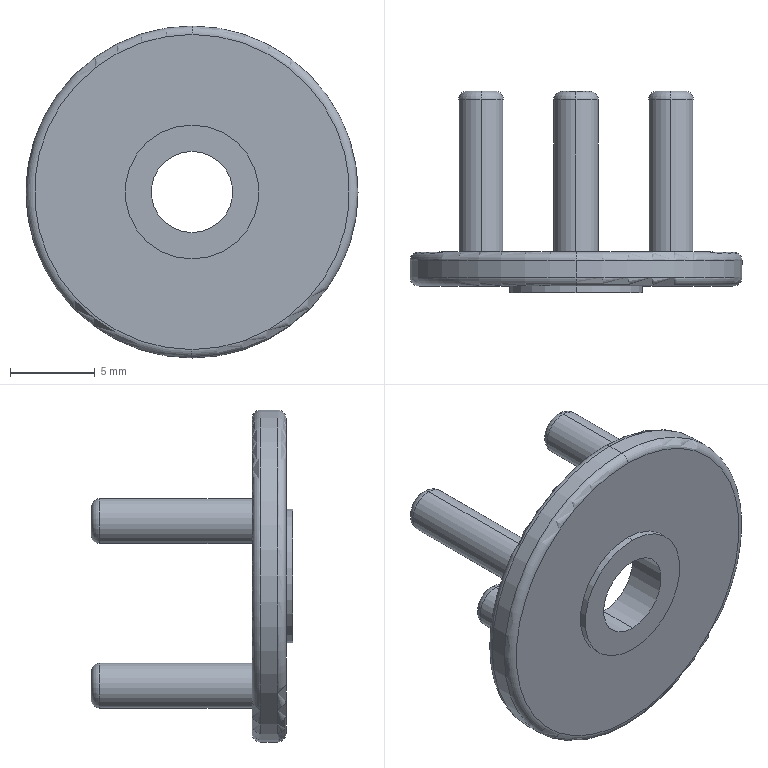Part | SolidWorks | features BaseBody 1 | 1 solid | 28 faces | box 19.6 x 11.9 x 19.6 mm | volume 729.046 mm3 | cylinder 12 | torus 10 | plane 6 | commonest cylinder face diameters 2.65 x6 4.8 x2 7.9 x2 19.6 x2
STEP:
#1=CARTESIAN_POINT('',(0.,0.,3.95));
#2=VERTEX_POINT('',#1);
#3=CARTESIAN_POINT('',(0.,0.,-3.95));
#4=VERTEX_POINT('',#3);
#5=CARTESIAN_POINT('',(0.,0.,0.));
#6=DIRECTION('',(0.,1.,0.));
#7=DIRECTION('',(0.,0.,1.));
#8=AXIS2_PLACEMENT_3D('',#5,#6,#7);
#9=CIRCLE('',#8,3.95);
#10=EDGE_CURVE('',#2,#4,#9,.T.);
#11=ORIENTED_EDGE('',*,*,#10,.F.);
#12=CARTESIAN_POINT('',(0.,-0.4,3.95));
#13=VERTEX_POINT('',#12);
#14=CARTESIAN_POINT('',(0.,-0.4,3.95));
#15=DIRECTION('',(0.,1.,0.));
#16=VECTOR('',#15,1000.);
#17=LINE('',#14,#16);
#18=EDGE_CURVE('',#13,#2,#17,.T.);
#19=ORIENTED_EDGE('',*,*,#18,.F.);
#20=CARTESIAN_POINT('',(0.,-0.4,-3.95));
#21=VERTEX_POINT('',#20);
#22=CARTESIAN_POINT('',(0.,-0.4,0.));
#23=DIRECTION('',(0.,-1.,0.));
#24=DIRECTION('',(0.,0.,-1.));
#25=AXIS2_PLACEMENT_3D('',#22,#23,#24);
#26=CIRCLE('',#25,3.95);
#27=EDGE_CURVE('',#21,#13,#26,.T.);
#28=ORIENTED_EDGE('',*,*,#27,.F.);
#29=CARTESIAN_POINT('',(0.,0.,-3.95));
#30=DIRECTION('',(0.,-1.,0.));
#31=VECTOR('',#30,1000.);
#32=LINE('',#29,#31);
#33=EDGE_CURVE('',#4,#21,#32,.T.);
#34=ORIENTED_EDGE('',*,*,#33,.F.);
#35=EDGE_LOOP('',(#11,#19,#28,#34));
#36=FACE_OUTER_BOUND('',#35,.T.);
#37=CARTESIAN_POINT('',(0.,-0.4,0.));
#38=DIRECTION('',(0.,1.,0.));
#39=DIRECTION('',(0.,0.,1.));
#40=AXIS2_PLACEMENT_3D('',#37,#38,#39);
#41=CYLINDRICAL_SURFACE('',#40,3.95);
#42=ADVANCED_FACE('',(#36),#41,.T.);
#43=ORIENTED_EDGE('',*,*,#33,.T.);
#44=CARTESIAN_POINT('',(0.,-0.4,0.));
#45=DIRECTION('',(0.,-1.,0.));
#46=DIRECTION('',(0.,0.,1.));
#47=AXIS2_PLACEMENT_3D('',#44,#45,#46);
#48=CIRCLE('',#47,3.95);
#49=EDGE_CURVE('',#13,#21,#48,.T.);
#50=ORIENTED_EDGE('',*,*,#49,.F.);
#51=ORIENTED_EDGE('',*,*,#18,.T.);
#52=CARTESIAN_POINT('',(0.,0.,0.));
#53=DIRECTION('',(0.,1.,0.));
#54=DIRECTION('',(0.,0.,-1.));
#55=AXIS2_PLACEMENT_3D('',#52,#53,#54);
#56=CIRCLE('',#55,3.95);
#57=EDGE_CURVE('',#4,#2,#56,.T.);
#58=ORIENTED_EDGE('',*,*,#57,.F.);
#59=EDGE_LOOP('',(#43,#50,#51,#58));
#60=FACE_OUTER_BOUND('',#59,.T.);
#61=CARTESIAN_POINT('',(0.,-0.4,0.));
#62=DIRECTION('',(0.,1.,0.));
#63=DIRECTION('',(0.,0.,1.));
#64=AXIS2_PLACEMENT_3D('',#61,#62,#63);
#65=CYLINDRICAL_SURFACE('',#64,3.95);
#66=ADVANCED_FACE('',(#60),#65,.T.);
#67=CARTESIAN_POINT('',(0.,-0.4,2.4));
#68=VERTEX_POINT('',#67);
#69=CARTESIAN_POINT('',(0.,-0.4,-2.4));
#70=VERTEX_POINT('',#69);
#71=CARTESIAN_POINT('',(0.,-0.4,0.));
#72=DIRECTION('',(0.,-1.,0.));
#73=DIRECTION('',(0.,0.,1.));
#74=AXIS2_PLACEMENT_3D('',#71,#72,#73);
#75=CIRCLE('',#74,2.4);
#76=EDGE_CURVE('',#68,#70,#75,.T.);
#77=ORIENTED_EDGE('',*,*,#76,.F.);
#78=CARTESIAN_POINT('',(0.,-0.4,0.));
#79=DIRECTION('',(0.,-1.,0.));
#80=DIRECTION('',(0.,0.,-1.));
#81=AXIS2_PLACEMENT_3D('',#78,#79,#80);
#82=CIRCLE('',#81,2.4);
#83=EDGE_CURVE('',#70,#68,#82,.T.);
#84=ORIENTED_EDGE('',*,*,#83,.F.);
#85=EDGE_LOOP('',(#77,#84));
#86=FACE_BOUND('',#85,.T.);
#87=ORIENTED_EDGE('',*,*,#27,.T.);
#88=ORIENTED_EDGE('',*,*,#49,.T.);
#89=EDGE_LOOP('',(#87,#88));
#90=FACE_OUTER_BOUND('',#89,.T.);
#91=CARTESIAN_POINT('',(0.,-0.4,0.));
#92=DIRECTION('',(0.,-1.,0.));
#93=DIRECTION('',(0.,0.,-1.));
#94=AXIS2_PLACEMENT_3D('',#91,#92,#93);
#95=PLANE('',#94);
#96=ADVANCED_FACE('',(#86,#90),#95,.T.);
#97=CARTESIAN_POINT('',(0.,2.,9.3));
#98=VERTEX_POINT('',#97);
#99=CARTESIAN_POINT('',(0.,2.,-9.3));
#100=VERTEX_POINT('',#99);
#101=CARTESIAN_POINT('',(0.,2.,0.));
#102=DIRECTION('',(0.,1.,0.));
#103=DIRECTION('',(0.,0.,1.));
#104=AXIS2_PLACEMENT_3D('',#101,#102,#103);
#105=CIRCLE('',#104,9.3);
#106=EDGE_CURVE('',#98,#100,#105,.T.);
#107=ORIENTED_EDGE('',*,*,#106,.F.);
#108=CARTESIAN_POINT('',(0.,1.5,9.8));
#109=VERTEX_POINT('',#108);
#110=CARTESIAN_POINT('',(0.,1.5,9.3));
#111=DIRECTION('',(-1.,0.,0.));
#112=DIRECTION('',(0.,0.,1.));
#113=AXIS2_PLACEMENT_3D('',#110,#111,#112);
#114=CIRCLE('',#113,0.5);
#115=EDGE_CURVE('',#109,#98,#114,.T.);
#116=ORIENTED_EDGE('',*,*,#115,.F.);
#117=CARTESIAN_POINT('',(0.,1.5,-9.8));
#118=VERTEX_POINT('',#117);
#119=CARTESIAN_POINT('',(0.,1.5,0.));
#120=DIRECTION('',(0.,-1.,0.));
#121=DIRECTION('',(0.,0.,-1.));
#122=AXIS2_PLACEMENT_3D('',#119,#120,#121);
#123=CIRCLE('',#122,9.8);
#124=EDGE_CURVE('',#118,#109,#123,.T.);
#125=ORIENTED_EDGE('',*,*,#124,.F.);
#126=CARTESIAN_POINT('',(0.,1.5,-9.3));
#127=DIRECTION('',(-1.,0.,0.));
#128=DIRECTION('',(0.,1.,0.));
#129=AXIS2_PLACEMENT_3D('',#126,#127,#128);
#130=CIRCLE('',#129,0.5);
#131=EDGE_CURVE('',#100,#118,#130,.T.);
#132=ORIENTED_EDGE('',*,*,#131,.F.);
#133=EDGE_LOOP('',(#107,#116,#125,#132));
#134=FACE_OUTER_BOUND('',#133,.T.);
#135=CARTESIAN_POINT('',(0.,1.5,0.));
#136=DIRECTION('',(0.,-1.,0.));
#137=DIRECTION('',(0.,0.,1.));
#138=AXIS2_PLACEMENT_3D('',#135,#136,#137);
#139=TOROIDAL_SURFACE('',#138,9.3,0.5);
#140=ADVANCED_FACE('',(#134),#139,.T.);
#141=ORIENTED_EDGE('',*,*,#131,.T.);
#142=CARTESIAN_POINT('',(0.,1.5,0.));
#143=DIRECTION('',(0.,-1.,0.));
#144=DIRECTION('',(0.,0.,1.));
#145=AXIS2_PLACEMENT_3D('',#142,#143,#144);
#146=CIRCLE('',#145,9.8);
#147=EDGE_CURVE('',#109,#118,#146,.T.);
#148=ORIENTED_EDGE('',*,*,#147,.F.);
#149=ORIENTED_EDGE('',*,*,#115,.T.);
#150=CARTESIAN_POINT('',(0.,2.,0.));
#151=DIRECTION('',(0.,1.,0.));
#152=DIRECTION('',(0.,0.,-1.));
#153=AXIS2_PLACEMENT_3D('',#150,#151,#152);
#154=CIRCLE('',#153,9.3);
#155=EDGE_CURVE('',#100,#98,#154,.T.);
#156=ORIENTED_EDGE('',*,*,#155,.F.);
#157=EDGE_LOOP('',(#141,#148,#149,#156));
#158=FACE_OUTER_BOUND('',#157,.T.);
#159=CARTESIAN_POINT('',(0.,1.5,0.));
#160=DIRECTION('',(0.,-1.,0.));
#161=DIRECTION('',(0.,0.,1.));
#162=AXIS2_PLACEMENT_3D('',#159,#160,#161);
#163=TOROIDAL_SURFACE('',#162,9.3,0.5);
#164=ADVANCED_FACE('',(#158),#163,.T.);
#165=CARTESIAN_POINT('',(0.,0.5,9.8));
#166=VERTEX_POINT('',#165);
#167=CARTESIAN_POINT('',(0.,0.5,-9.8));
#168=VERTEX_POINT('',#167);
#169=CARTESIAN_POINT('',(0.,0.5,0.));
#170=DIRECTION('',(0.,1.,0.));
#171=DIRECTION('',(0.,0.,1.));
#172=AXIS2_PLACEMENT_3D('',#169,#170,#171);
#173=CIRCLE('',#172,9.8);
#174=EDGE_CURVE('',#166,#168,#173,.T.);
#175=ORIENTED_EDGE('',*,*,#174,.F.);
#176=CARTESIAN_POINT('',(0.,0.,9.3));
#177=VERTEX_POINT('',#176);
#178=CARTESIAN_POINT('',(0.,0.5,9.3));
#179=DIRECTION('',(-1.,0.,0.));
#180=DIRECTION('',(0.,-1.,0.00001628));
#181=AXIS2_PLACEMENT_3D('',#178,#179,#180);
#182=CIRCLE('',#181,0.5);
#183=EDGE_CURVE('',#177,#166,#182,.T.);
#184=ORIENTED_EDGE('',*,*,#183,.F.);
#185=CARTESIAN_POINT('',(0.,0.,-9.3));
#186=VERTEX_POINT('',#185);
#187=CARTESIAN_POINT('',(0.,0.,0.));
#188=DIRECTION('',(0.,-1.,0.));
#189=DIRECTION('',(0.,0.,-1.));
#190=AXIS2_PLACEMENT_3D('',#187,#188,#189);
#191=CIRCLE('',#190,9.3);
#192=EDGE_CURVE('',#186,#177,#191,.T.);
#193=ORIENTED_EDGE('',*,*,#192,.F.);
#194=CARTESIAN_POINT('',(0.,0.5,-9.3));
#195=DIRECTION('',(-1.,0.,0.));
#196=DIRECTION('',(0.,0.,-1.));
#197=AXIS2_PLACEMENT_3D('',#194,#195,#196);
#198=CIRCLE('',#197,0.5);
#199=EDGE_CURVE('',#168,#186,#198,.T.);
#200=ORIENTED_EDGE('',*,*,#199,.F.);
#201=EDGE_LOOP('',(#175,#184,#193,#200));
#202=FACE_OUTER_BOUND('',#201,.T.);
#203=CARTESIAN_POINT('',(0.,0.5,0.));
#204=DIRECTION('',(0.,-1.,0.));
#205=DIRECTION('',(0.,0.,1.));
#206=AXIS2_PLACEMENT_3D('',#203,#204,#205);
#207=TOROIDAL_SURFACE('',#206,9.3,0.5);
#208=ADVANCED_FACE('',(#202),#207,.T.);
#209=CARTESIAN_POINT('',(0.,0.5,0.));
#210=DIRECTION('',(0.,1.,0.));
#211=DIRECTION('',(0.,0.,-1.));
#212=AXIS2_PLACEMENT_3D('',#209,#210,#211);
#213=CIRCLE('',#212,9.8);
#214=EDGE_CURVE('',#168,#166,#213,.T.);
#215=ORIENTED_EDGE('',*,*,#214,.F.);
#216=ORIENTED_EDGE('',*,*,#199,.T.);
#217=CARTESIAN_POINT('',(0.,0.,0.));
#218=DIRECTION('',(0.,-1.,0.));
#219=DIRECTION('',(0.,0.,1.));
#220=AXIS2_PLACEMENT_3D('',#217,#218,#219);
#221=CIRCLE('',#220,9.3);
#222=EDGE_CURVE('',#177,#186,#221,.T.);
#223=ORIENTED_EDGE('',*,*,#222,.F.);
#224=ORIENTED_EDGE('',*,*,#183,.T.);
#225=EDGE_LOOP('',(#215,#216,#223,#224));
#226=FACE_OUTER_BOUND('',#225,.T.);
#227=CARTESIAN_POINT('',(0.,0.5,0.));
#228=DIRECTION('',(0.,-1.,0.));
#229=DIRECTION('',(0.,0.,1.));
#230=AXIS2_PLACEMENT_3D('',#227,#228,#229);
#231=TOROIDAL_SURFACE('',#230,9.3,0.5);
#232=ADVANCED_FACE('',(#226),#231,.T.);
#233=CARTESIAN_POINT('',(-5.608,11.5,4.062));
#234=VERTEX_POINT('',#233);
#235=CARTESIAN_POINT('',(-5.608,11.5,2.413));
#236=VERTEX_POINT('',#235);
#237=CARTESIAN_POINT('',(-5.608,11.5,3.237));
#238=DIRECTION('',(0.,1.,0.));
#239=DIRECTION('',(-0.000000017,0.,1.));
#240=AXIS2_PLACEMENT_3D('',#237,#238,#239);
#241=CIRCLE('',#240,0.825);
#242=EDGE_CURVE('',#234,#236,#241,.T.);
#243=ORIENTED_EDGE('',*,*,#242,.F.);
#244=CARTESIAN_POINT('',(-5.608,11.,4.562));
#245=VERTEX_POINT('',#244);
#246=CARTESIAN_POINT('',(-5.608,11.,4.062));
#247=DIRECTION('',(-1.,0.,0.));
#248=DIRECTION('',(0.,0.,1.));
#249=AXIS2_PLACEMENT_3D('',#246,#247,#248);
#250=CIRCLE('',#249,0.5);
#251=EDGE_CURVE('',#245,#234,#250,.T.);
#252=ORIENTED_EDGE('',*,*,#251,.F.);
#253=CARTESIAN_POINT('',(-5.608,11.,1.912));
#254=VERTEX_POINT('',#253);
#255=CARTESIAN_POINT('',(-5.608,11.,3.237));
#256=DIRECTION('',(0.,-1.,0.));
#257=DIRECTION('',(0.,0.,-1.));
#258=AXIS2_PLACEMENT_3D('',#255,#256,#257);
#259=CIRCLE('',#258,1.325);
#260=EDGE_CURVE('',#254,#245,#259,.T.);
#261=ORIENTED_EDGE('',*,*,#260,.F.);
#262=CARTESIAN_POINT('',(-5.608,11.,2.413));
#263=DIRECTION('',(-1.,0.,0.));
#264=DIRECTION('',(0.,1.,0.));
#265=AXIS2_PLACEMENT_3D('',#262,#263,#264);
#266=CIRCLE('',#265,0.5);
#267=EDGE_CURVE('',#236,#254,#266,.T.);
#268=ORIENTED_EDGE('',*,*,#267,.F.);
#269=EDGE_LOOP('',(#243,#252,#261,#268));
#270=FACE_OUTER_BOUND('',#269,.T.);
#271=CARTESIAN_POINT('',(-5.608,11.,3.237));
#272=DIRECTION('',(0.,-1.,0.));
#273=DIRECTION('',(0.,0.,1.));
#274=AXIS2_PLACEMENT_3D('',#271,#272,#273);
#275=TOROIDAL_SURFACE('',#274,0.825,0.5);
#276=ADVANCED_FACE('',(#270),#275,.T.);
#277=ORIENTED_EDGE('',*,*,#267,.T.);
#278=CARTESIAN_POINT('',(-5.608,11.,3.237));
#279=DIRECTION('',(0.,-1.,0.));
#280=DIRECTION('',(0.,0.,1.));
#281=AXIS2_PLACEMENT_3D('',#278,#279,#280);
#282=CIRCLE('',#281,1.325);
#283=EDGE_CURVE('',#245,#254,#282,.T.);
#284=ORIENTED_EDGE('',*,*,#283,.F.);
#285=ORIENTED_EDGE('',*,*,#251,.T.);
#286=CARTESIAN_POINT('',(-5.608,11.5,3.237));
#287=DIRECTION('',(0.,1.,0.));
#288=DIRECTION('',(0.,0.,-1.));
#289=AXIS2_PLACEMENT_3D('',#286,#287,#288);
#290=CIRCLE('',#289,0.825);
#291=EDGE_CURVE('',#236,#234,#290,.T.);
#292=ORIENTED_EDGE('',*,*,#291,.F.);
#293=EDGE_LOOP('',(#277,#284,#285,#292));
#294=FACE_OUTER_BOUND('',#293,.T.);
#295=CARTESIAN_POINT('',(-5.608,11.,3.237));
#296=DIRECTION('',(0.,-1.,0.));
#297=DIRECTION('',(0.,0.,1.));
#298=AXIS2_PLACEMENT_3D('',#295,#296,#297);
#299=TOROIDAL_SURFACE('',#298,0.825,0.5);
#300=ADVANCED_FACE('',(#294),#299,.T.);
#301=CARTESIAN_POINT('',(-0.000000007,11.5,-5.65));
#302=VERTEX_POINT('',#301);
#303=CARTESIAN_POINT('',(0.,11.5,-7.3));
#304=VERTEX_POINT('',#303);
#305=CARTESIAN_POINT('',(0.,11.5,-6.475));
#306=DIRECTION('',(0.,1.,0.));
#307=DIRECTION('',(-0.000000017,0.,1.));
#308=AXIS2_PLACEMENT_3D('',#305,#306,#307);
#309=CIRCLE('',#308,0.825);
#310=EDGE_CURVE('',#302,#304,#309,.T.);
#311=ORIENTED_EDGE('',*,*,#310,.F.);
#312=CARTESIAN_POINT('',(0.,11.,-5.15));
#313=VERTEX_POINT('',#312);
#314=CARTESIAN_POINT('',(0.,11.,-5.65));
#315=DIRECTION('',(-1.,0.,0.));
#316=DIRECTION('',(0.,0.,1.));
#317=AXIS2_PLACEMENT_3D('',#314,#315,#316);
#318=CIRCLE('',#317,0.5);
#319=EDGE_CURVE('',#313,#302,#318,.T.);
#320=ORIENTED_EDGE('',*,*,#319,.F.);
#321=CARTESIAN_POINT('',(0.,11.,-7.8));
#322=VERTEX_POINT('',#321);
#323=CARTESIAN_POINT('',(0.,11.,-6.475));
#324=DIRECTION('',(0.,-1.,0.));
#325=DIRECTION('',(0.,0.,-1.));
#326=AXIS2_PLACEMENT_3D('',#323,#324,#325);
#327=CIRCLE('',#326,1.325);
#328=EDGE_CURVE('',#322,#313,#327,.T.);
#329=ORIENTED_EDGE('',*,*,#328,.F.);
#330=CARTESIAN_POINT('',(0.,11.,-7.3));
#331=DIRECTION('',(-1.,0.,0.));
#332=DIRECTION('',(0.,1.,0.));
#333=AXIS2_PLACEMENT_3D('',#330,#331,#332);
#334=CIRCLE('',#333,0.5);
#335=EDGE_CURVE('',#304,#322,#334,.T.);
#336=ORIENTED_EDGE('',*,*,#335,.F.);
#337=EDGE_LOOP('',(#311,#320,#329,#336));
#338=FACE_OUTER_BOUND('',#337,.T.);
#339=CARTESIAN_POINT('',(0.,11.,-6.475));
#340=DIRECTION('',(0.,-1.,0.));
#341=DIRECTION('',(0.,0.,1.));
#342=AXIS2_PLACEMENT_3D('',#339,#340,#341);
#343=TOROIDAL_SURFACE('',#342,0.825,0.5);
#344=ADVANCED_FACE('',(#338),#343,.T.);
#345=ORIENTED_EDGE('',*,*,#335,.T.);
#346=CARTESIAN_POINT('',(0.,11.,-6.475));
#347=DIRECTION('',(0.,-1.,0.));
#348=DIRECTION('',(0.,0.,1.));
#349=AXIS2_PLACEMENT_3D('',#346,#347,#348);
#350=CIRCLE('',#349,1.325);
#351=EDGE_CURVE('',#313,#322,#350,.T.);
#352=ORIENTED_EDGE('',*,*,#351,.F.);
#353=ORIENTED_EDGE('',*,*,#319,.T.);
#354=CARTESIAN_POINT('',(0.,11.5,-6.475));
#355=DIRECTION('',(0.,1.,0.));
#356=DIRECTION('',(0.,0.,-1.));
#357=AXIS2_PLACEMENT_3D('',#354,#355,#356);
#358=CIRCLE('',#357,0.825);
#359=EDGE_CURVE('',#304,#302,#358,.T.);
#360=ORIENTED_EDGE('',*,*,#359,.F.);
#361=EDGE_LOOP('',(#345,#352,#353,#360));
#362=FACE_OUTER_BOUND('',#361,.T.);
#363=CARTESIAN_POINT('',(0.,11.,-6.475));
#364=DIRECTION('',(0.,-1.,0.));
#365=DIRECTION('',(0.,0.,1.));
#366=AXIS2_PLACEMENT_3D('',#363,#364,#365);
#367=TOROIDAL_SURFACE('',#366,0.825,0.5);
#368=ADVANCED_FACE('',(#362),#367,.T.);
#369=CARTESIAN_POINT('',(5.608,11.5,4.062));
#370=VERTEX_POINT('',#369);
#371=CARTESIAN_POINT('',(5.608,11.5,2.413));
#372=VERTEX_POINT('',#371);
#373=CARTESIAN_POINT('',(5.608,11.5,3.237));
#374=DIRECTION('',(0.,1.,0.));
#375=DIRECTION('',(-0.000000017,0.,1.));
#376=AXIS2_PLACEMENT_3D('',#373,#374,#375);
#377=CIRCLE('',#376,0.825);
#378=EDGE_CURVE('',#370,#372,#377,.T.);
#379=ORIENTED_EDGE('',*,*,#378,.F.);
#380=CARTESIAN_POINT('',(5.608,11.,4.562));
#381=VERTEX_POINT('',#380);
#382=CARTESIAN_POINT('',(5.608,11.,4.062));
#383=DIRECTION('',(-1.,0.,0.));
#384=DIRECTION('',(0.,0.,1.));
#385=AXIS2_PLACEMENT_3D('',#382,#383,#384);
#386=CIRCLE('',#385,0.5);
#387=EDGE_CURVE('',#381,#370,#386,.T.);
#388=ORIENTED_EDGE('',*,*,#387,.F.);
#389=CARTESIAN_POINT('',(5.608,11.,1.912));
#390=VERTEX_POINT('',#389);
#391=CARTESIAN_POINT('',(5.608,11.,3.237));
#392=DIRECTION('',(0.,-1.,0.));
#393=DIRECTION('',(0.,0.,-1.));
#394=AXIS2_PLACEMENT_3D('',#391,#392,#393);
#395=CIRCLE('',#394,1.325);
#396=EDGE_CURVE('',#390,#381,#395,.T.);
#397=ORIENTED_EDGE('',*,*,#396,.F.);
#398=CARTESIAN_POINT('',(5.608,11.,2.413));
#399=DIRECTION('',(-1.,0.,0.));
#400=DIRECTION('',(0.,1.,0.));
#401=AXIS2_PLACEMENT_3D('',#398,#399,#400);
#402=CIRCLE('',#401,0.5);
#403=EDGE_CURVE('',#372,#390,#402,.T.);
#404=ORIENTED_EDGE('',*,*,#403,.F.);
#405=EDGE_LOOP('',(#379,#388,#397,#404));
#406=FACE_OUTER_BOUND('',#405,.T.);
#407=CARTESIAN_POINT('',(5.608,11.,3.237));
#408=DIRECTION('',(0.,-1.,0.));
#409=DIRECTION('',(0.,0.,1.));
#410=AXIS2_PLACEMENT_3D('',#407,#408,#409);
#411=TOROIDAL_SURFACE('',#410,0.825,0.5);
#412=ADVANCED_FACE('',(#406),#411,.T.);
#413=ORIENTED_EDGE('',*,*,#403,.T.);
#414=CARTESIAN_POINT('',(5.608,11.,3.237));
#415=DIRECTION('',(0.,-1.,0.));
#416=DIRECTION('',(0.,0.,1.));
#417=AXIS2_PLACEMENT_3D('',#414,#415,#416);
#418=CIRCLE('',#417,1.325);
#419=EDGE_CURVE('',#381,#390,#418,.T.);
#420=ORIENTED_EDGE('',*,*,#419,.F.);
#421=ORIENTED_EDGE('',*,*,#387,.T.);
#422=CARTESIAN_POINT('',(5.608,11.5,3.237));
#423=DIRECTION('',(0.,1.,0.));
#424=DIRECTION('',(0.,0.,-1.));
#425=AXIS2_PLACEMENT_3D('',#422,#423,#424);
#426=CIRCLE('',#425,0.825);
#427=EDGE_CURVE('',#372,#370,#426,.T.);
#428=ORIENTED_EDGE('',*,*,#427,.F.);
#429=EDGE_LOOP('',(#413,#420,#421,#428));
#430=FACE_OUTER_BOUND('',#429,.T.);
#431=CARTESIAN_POINT('',(5.608,11.,3.237));
#432=DIRECTION('',(0.,-1.,0.));
#433=DIRECTION('',(0.,0.,1.));
#434=AXIS2_PLACEMENT_3D('',#431,#432,#433);
#435=TOROIDAL_SURFACE('',#434,0.825,0.5);
#436=ADVANCED_FACE('',(#430),#435,.T.);
#437=ORIENTED_EDGE('',*,*,#427,.T.);
#438=ORIENTED_EDGE('',*,*,#378,.T.);
#439=EDGE_LOOP('',(#437,#438));
#440=FACE_OUTER_BOUND('',#439,.T.);
#441=CARTESIAN_POINT('',(5.608,11.5,3.237));
#442=DIRECTION('',(0.,1.,0.));
#443=DIRECTION('',(1.,0.,0.));
#444=AXIS2_PLACEMENT_3D('',#441,#442,#443);
#445=PLANE('',#444);
#446=ADVANCED_FACE('',(#440),#445,.T.);
#447=CARTESIAN_POINT('',(5.608,2.,1.912));
#448=VERTEX_POINT('',#447);
#449=CARTESIAN_POINT('',(5.608,2.,4.562));
#450=VERTEX_POINT('',#449);
#451=CARTESIAN_POINT('',(5.608,2.,3.237));
#452=DIRECTION('',(0.,-1.,0.));
#453=DIRECTION('',(0.,0.,-1.));
#454=AXIS2_PLACEMENT_3D('',#451,#452,#453);
#455=CIRCLE('',#454,1.325);
#456=EDGE_CURVE('',#448,#450,#455,.T.);
#457=ORIENTED_EDGE('',*,*,#456,.F.);
#458=CARTESIAN_POINT('',(5.608,11.,1.912));
#459=DIRECTION('',(0.,-1.,0.));
#460=VECTOR('',#459,1000.);
#461=LINE('',#458,#460);
#462=EDGE_CURVE('',#390,#448,#461,.T.);
#463=ORIENTED_EDGE('',*,*,#462,.F.);
#464=ORIENTED_EDGE('',*,*,#396,.T.);
#465=CARTESIAN_POINT('',(5.608,2.,4.562));
#466=DIRECTION('',(0.,1.,0.));
#467=VECTOR('',#466,1000.);
#468=LINE('',#465,#467);
#469=EDGE_CURVE('',#450,#381,#468,.T.);
#470=ORIENTED_EDGE('',*,*,#469,.F.);
#471=EDGE_LOOP('',(#457,#463,#464,#470));
#472=FACE_OUTER_BOUND('',#471,.T.);
#473=CARTESIAN_POINT('',(5.608,11.,3.237));
#474=DIRECTION('',(0.,-1.,0.));
#475=DIRECTION('',(0.,0.,-1.));
#476=AXIS2_PLACEMENT_3D('',#473,#474,#475);
#477=CYLINDRICAL_SURFACE('',#476,1.325);
#478=ADVANCED_FACE('',(#472),#477,.T.);
#479=ORIENTED_EDGE('',*,*,#469,.T.);
#480=ORIENTED_EDGE('',*,*,#419,.T.);
#481=ORIENTED_EDGE('',*,*,#462,.T.);
#482=CARTESIAN_POINT('',(5.608,2.,3.237));
#483=DIRECTION('',(0.,-1.,0.));
#484=DIRECTION('',(0.,0.,1.));
#485=AXIS2_PLACEMENT_3D('',#482,#483,#484);
#486=CIRCLE('',#485,1.325);
#487=EDGE_CURVE('',#450,#448,#486,.T.);
#488=ORIENTED_EDGE('',*,*,#487,.F.);
#489=EDGE_LOOP('',(#479,#480,#481,#488));
#490=FACE_OUTER_BOUND('',#489,.T.);
#491=CARTESIAN_POINT('',(5.608,11.,3.237));
#492=DIRECTION('',(0.,-1.,0.));
#493=DIRECTION('',(0.,0.,-1.));
#494=AXIS2_PLACEMENT_3D('',#491,#492,#493);
#495=CYLINDRICAL_SURFACE('',#494,1.325);
#496=ADVANCED_FACE('',(#490),#495,.T.);
#497=ORIENTED_EDGE('',*,*,#291,.T.);
#498=ORIENTED_EDGE('',*,*,#242,.T.);
#499=EDGE_LOOP('',(#497,#498));
#500=FACE_OUTER_BOUND('',#499,.T.);
#501=CARTESIAN_POINT('',(-5.608,11.5,3.237));
#502=DIRECTION('',(0.,1.,0.));
#503=DIRECTION('',(1.,0.,0.));
#504=AXIS2_PLACEMENT_3D('',#501,#502,#503);
#505=PLANE('',#504);
#506=ADVANCED_FACE('',(#500),#505,.T.);
#507=CARTESIAN_POINT('',(-5.608,2.,1.912));
#508=VERTEX_POINT('',#507);
#509=CARTESIAN_POINT('',(-5.608,2.,4.562));
#510=VERTEX_POINT('',#509);
#511=CARTESIAN_POINT('',(-5.608,2.,3.237));
#512=DIRECTION('',(0.,-1.,0.));
#513=DIRECTION('',(0.,0.,-1.));
#514=AXIS2_PLACEMENT_3D('',#511,#512,#513);
#515=CIRCLE('',#514,1.325);
#516=EDGE_CURVE('',#508,#510,#515,.T.);
#517=ORIENTED_EDGE('',*,*,#516,.F.);
#518=CARTESIAN_POINT('',(-5.608,11.,1.912));
#519=DIRECTION('',(0.,-1.,0.));
#520=VECTOR('',#519,1000.);
#521=LINE('',#518,#520);
#522=EDGE_CURVE('',#254,#508,#521,.T.);
#523=ORIENTED_EDGE('',*,*,#522,.F.);
#524=ORIENTED_EDGE('',*,*,#260,.T.);
#525=CARTESIAN_POINT('',(-5.608,2.,4.562));
#526=DIRECTION('',(0.,1.,0.));
#527=VECTOR('',#526,1000.);
#528=LINE('',#525,#527);
#529=EDGE_CURVE('',#510,#245,#528,.T.);
#530=ORIENTED_EDGE('',*,*,#529,.F.);
#531=EDGE_LOOP('',(#517,#523,#524,#530));
#532=FACE_OUTER_BOUND('',#531,.T.);
#533=CARTESIAN_POINT('',(-5.608,11.,3.237));
#534=DIRECTION('',(0.,-1.,0.));
#535=DIRECTION('',(0.,0.,-1.));
#536=AXIS2_PLACEMENT_3D('',#533,#534,#535);
#537=CYLINDRICAL_SURFACE('',#536,1.325);
#538=ADVANCED_FACE('',(#532),#537,.T.);
#539=ORIENTED_EDGE('',*,*,#529,.T.);
#540=ORIENTED_EDGE('',*,*,#283,.T.);
#541=ORIENTED_EDGE('',*,*,#522,.T.);
#542=CARTESIAN_POINT('',(-5.608,2.,3.237));
#543=DIRECTION('',(0.,-1.,0.));
#544=DIRECTION('',(0.,0.,1.));
#545=AXIS2_PLACEMENT_3D('',#542,#543,#544);
#546=CIRCLE('',#545,1.325);
#547=EDGE_CURVE('',#510,#508,#546,.T.);
#548=ORIENTED_EDGE('',*,*,#547,.F.);
#549=EDGE_LOOP('',(#539,#540,#541,#548));
#550=FACE_OUTER_BOUND('',#549,.T.);
#551=CARTESIAN_POINT('',(-5.608,11.,3.237));
#552=DIRECTION('',(0.,-1.,0.));
#553=DIRECTION('',(0.,0.,-1.));
#554=AXIS2_PLACEMENT_3D('',#551,#552,#553);
#555=CYLINDRICAL_SURFACE('',#554,1.325);
#556=ADVANCED_FACE('',(#550),#555,.T.);
#557=ORIENTED_EDGE('',*,*,#359,.T.);
#558=ORIENTED_EDGE('',*,*,#310,.T.);
#559=EDGE_LOOP('',(#557,#558));
#560=FACE_OUTER_BOUND('',#559,.T.);
#561=CARTESIAN_POINT('',(0.,11.5,-6.475));
#562=DIRECTION('',(0.,1.,0.));
#563=DIRECTION('',(1.,0.,0.));
#564=AXIS2_PLACEMENT_3D('',#561,#562,#563);
#565=PLANE('',#564);
#566=ADVANCED_FACE('',(#560),#565,.T.);
#567=CARTESIAN_POINT('',(0.,2.,-7.8));
#568=VERTEX_POINT('',#567);
#569=CARTESIAN_POINT('',(0.,2.,-5.15));
#570=VERTEX_POINT('',#569);
#571=CARTESIAN_POINT('',(0.,2.,-6.475));
#572=DIRECTION('',(0.,-1.,0.));
#573=DIRECTION('',(0.,0.,-1.));
#574=AXIS2_PLACEMENT_3D('',#571,#572,#573);
#575=CIRCLE('',#574,1.325);
#576=EDGE_CURVE('',#568,#570,#575,.T.);
#577=ORIENTED_EDGE('',*,*,#576,.F.);
#578=CARTESIAN_POINT('',(0.,11.,-7.8));
#579=DIRECTION('',(0.,-1.,0.));
#580=VECTOR('',#579,1000.);
#581=LINE('',#578,#580);
#582=EDGE_CURVE('',#322,#568,#581,.T.);
#583=ORIENTED_EDGE('',*,*,#582,.F.);
#584=ORIENTED_EDGE('',*,*,#328,.T.);
#585=CARTESIAN_POINT('',(0.,2.,-5.15));
#586=DIRECTION('',(0.,1.,0.));
#587=VECTOR('',#586,1000.);
#588=LINE('',#585,#587);
#589=EDGE_CURVE('',#570,#313,#588,.T.);
#590=ORIENTED_EDGE('',*,*,#589,.F.);
#591=EDGE_LOOP('',(#577,#583,#584,#590));
#592=FACE_OUTER_BOUND('',#591,.T.);
#593=CARTESIAN_POINT('',(0.,11.,-6.475));
#594=DIRECTION('',(0.,-1.,0.));
#595=DIRECTION('',(0.,0.,-1.));
#596=AXIS2_PLACEMENT_3D('',#593,#594,#595);
#597=CYLINDRICAL_SURFACE('',#596,1.325);
#598=ADVANCED_FACE('',(#592),#597,.T.);
#599=ORIENTED_EDGE('',*,*,#589,.T.);
#600=ORIENTED_EDGE('',*,*,#351,.T.);
#601=ORIENTED_EDGE('',*,*,#582,.T.);
#602=CARTESIAN_POINT('',(0.,2.,-6.475));
#603=DIRECTION('',(0.,-1.,0.));
#604=DIRECTION('',(0.,0.,1.));
#605=AXIS2_PLACEMENT_3D('',#602,#603,#604);
#606=CIRCLE('',#605,1.325);
#607=EDGE_CURVE('',#570,#568,#606,.T.);
#608=ORIENTED_EDGE('',*,*,#607,.F.);
#609=EDGE_LOOP('',(#599,#600,#601,#608));
#610=FACE_OUTER_BOUND('',#609,.T.);
#611=CARTESIAN_POINT('',(0.,11.,-6.475));
#612=DIRECTION('',(0.,-1.,0.));
#613=DIRECTION('',(0.,0.,-1.));
#614=AXIS2_PLACEMENT_3D('',#611,#612,#613);
#615=CYLINDRICAL_SURFACE('',#614,1.325);
#616=ADVANCED_FACE('',(#610),#615,.T.);
#617=ORIENTED_EDGE('',*,*,#83,.T.);
#618=CARTESIAN_POINT('',(0.,2.,2.4));
#619=VERTEX_POINT('',#618);
#620=CARTESIAN_POINT('',(0.,2.,2.4));
#621=DIRECTION('',(0.,-1.,0.));
#622=VECTOR('',#621,1000.);
#623=LINE('',#620,#622);
#624=EDGE_CURVE('',#619,#68,#623,.T.);
#625=ORIENTED_EDGE('',*,*,#624,.F.);
#626=CARTESIAN_POINT('',(0.,2.,-2.4));
#627=VERTEX_POINT('',#626);
#628=CARTESIAN_POINT('',(0.,2.,0.));
#629=DIRECTION('',(0.,-1.,0.));
#630=DIRECTION('',(0.,0.,-1.));
#631=AXIS2_PLACEMENT_3D('',#628,#629,#630);
#632=CIRCLE('',#631,2.4);
#633=EDGE_CURVE('',#627,#619,#632,.T.);
#634=ORIENTED_EDGE('',*,*,#633,.F.);
#635=CARTESIAN_POINT('',(0.,-0.4,-2.4));
#636=DIRECTION('',(0.,1.,0.));
#637=VECTOR('',#636,1000.);
#638=LINE('',#635,#637);
#639=EDGE_CURVE('',#70,#627,#638,.T.);
#640=ORIENTED_EDGE('',*,*,#639,.F.);
#641=EDGE_LOOP('',(#617,#625,#634,#640));
#642=FACE_OUTER_BOUND('',#641,.T.);
#643=CARTESIAN_POINT('',(0.,-0.4,0.));
#644=DIRECTION('',(0.,1.,0.));
#645=DIRECTION('',(0.,0.,1.));
#646=AXIS2_PLACEMENT_3D('',#643,#644,#645);
#647=CYLINDRICAL_SURFACE('',#646,2.4);
#648=ADVANCED_FACE('',(#642),#647,.F.);
#649=ORIENTED_EDGE('',*,*,#639,.T.);
#650=CARTESIAN_POINT('',(0.,2.,0.));
#651=DIRECTION('',(0.,-1.,0.));
#652=DIRECTION('',(0.,0.,1.));
#653=AXIS2_PLACEMENT_3D('',#650,#651,#652);
#654=CIRCLE('',#653,2.4);
#655=EDGE_CURVE('',#619,#627,#654,.T.);
#656=ORIENTED_EDGE('',*,*,#655,.F.);
#657=ORIENTED_EDGE('',*,*,#624,.T.);
#658=ORIENTED_EDGE('',*,*,#76,.T.);
#659=EDGE_LOOP('',(#649,#656,#657,#658));
#660=FACE_OUTER_BOUND('',#659,.T.);
#661=CARTESIAN_POINT('',(0.,-0.4,0.));
#662=DIRECTION('',(0.,1.,0.));
#663=DIRECTION('',(0.,0.,1.));
#664=AXIS2_PLACEMENT_3D('',#661,#662,#663);
#665=CYLINDRICAL_SURFACE('',#664,2.4);
#666=ADVANCED_FACE('',(#660),#665,.F.);
#667=ORIENTED_EDGE('',*,*,#174,.T.);
#668=CARTESIAN_POINT('',(0.,1.5,-9.8));
#669=DIRECTION('',(0.,-1.,0.));
#670=VECTOR('',#669,1000.);
#671=LINE('',#668,#670);
#672=EDGE_CURVE('',#118,#168,#671,.T.);
#673=ORIENTED_EDGE('',*,*,#672,.F.);
#674=ORIENTED_EDGE('',*,*,#124,.T.);
#675=CARTESIAN_POINT('',(0.,0.5,9.8));
#676=DIRECTION('',(0.,1.,0.));
#677=VECTOR('',#676,1000.);
#678=LINE('',#675,#677);
#679=EDGE_CURVE('',#166,#109,#678,.T.);
#680=ORIENTED_EDGE('',*,*,#679,.F.);
#681=EDGE_LOOP('',(#667,#673,#674,#680));
#682=FACE_OUTER_BOUND('',#681,.T.);
#683=CARTESIAN_POINT('',(0.,1.5,0.));
#684=DIRECTION('',(0.,-1.,0.));
#685=DIRECTION('',(0.,0.,-1.));
#686=AXIS2_PLACEMENT_3D('',#683,#684,#685);
#687=CYLINDRICAL_SURFACE('',#686,9.8);
#688=ADVANCED_FACE('',(#682),#687,.T.);
#689=ORIENTED_EDGE('',*,*,#214,.T.);
#690=ORIENTED_EDGE('',*,*,#679,.T.);
#691=ORIENTED_EDGE('',*,*,#147,.T.);
#692=ORIENTED_EDGE('',*,*,#672,.T.);
#693=EDGE_LOOP('',(#689,#690,#691,#692));
#694=FACE_OUTER_BOUND('',#693,.T.);
#695=CARTESIAN_POINT('',(0.,1.5,0.));
#696=DIRECTION('',(0.,-1.,0.));
#697=DIRECTION('',(0.,0.,-1.));
#698=AXIS2_PLACEMENT_3D('',#695,#696,#697);
#699=CYLINDRICAL_SURFACE('',#698,9.8);
#700=ADVANCED_FACE('',(#694),#699,.T.);
#701=ORIENTED_EDGE('',*,*,#547,.T.);
#702=ORIENTED_EDGE('',*,*,#516,.T.);
#703=EDGE_LOOP('',(#701,#702));
#704=FACE_BOUND('',#703,.T.);
#705=ORIENTED_EDGE('',*,*,#633,.T.);
#706=ORIENTED_EDGE('',*,*,#655,.T.);
#707=EDGE_LOOP('',(#705,#706));
#708=FACE_BOUND('',#707,.T.);
#709=ORIENTED_EDGE('',*,*,#607,.T.);
#710=ORIENTED_EDGE('',*,*,#576,.T.);
#711=EDGE_LOOP('',(#709,#710));
#712=FACE_BOUND('',#711,.T.);
#713=ORIENTED_EDGE('',*,*,#487,.T.);
#714=ORIENTED_EDGE('',*,*,#456,.T.);
#715=EDGE_LOOP('',(#713,#714));
#716=FACE_BOUND('',#715,.T.);
#717=ORIENTED_EDGE('',*,*,#155,.T.);
#718=ORIENTED_EDGE('',*,*,#106,.T.);
#719=EDGE_LOOP('',(#717,#718));
#720=FACE_OUTER_BOUND('',#719,.T.);
#721=CARTESIAN_POINT('',(0.,2.,0.));
#722=DIRECTION('',(0.,1.,0.));
#723=DIRECTION('',(1.,0.,0.));
#724=AXIS2_PLACEMENT_3D('',#721,#722,#723);
#725=PLANE('',#724);
#726=ADVANCED_FACE('',(#704,#708,#712,#716,#720),#725,.T.);
#727=ORIENTED_EDGE('',*,*,#57,.T.);
#728=ORIENTED_EDGE('',*,*,#10,.T.);
#729=EDGE_LOOP('',(#727,#728));
#730=FACE_BOUND('',#729,.T.);
#731=ORIENTED_EDGE('',*,*,#192,.T.);
#732=ORIENTED_EDGE('',*,*,#222,.T.);
#733=EDGE_LOOP('',(#731,#732));
#734=FACE_OUTER_BOUND('',#733,.T.);
#735=CARTESIAN_POINT('',(0.,0.,0.));
#736=DIRECTION('',(0.,-1.,0.));
#737=DIRECTION('',(0.,0.,-1.));
#738=AXIS2_PLACEMENT_3D('',#735,#736,#737);
#739=PLANE('',#738);
#740=ADVANCED_FACE('',(#730,#734),#739,.T.);
#741=CLOSED_SHELL('',(#42,#66,#96,#140,#164,#208,#232,#276,#300,#344,#368,#412,#436,#446,#478,#496,#506,#538,#556,#566,#598,#616,#648,#666,#688,#700,#726,#740));
#742=MANIFOLD_SOLID_BREP('',#741);
#743=CARTESIAN_POINT('',(0.,0.,0.));
#744=DIRECTION('',(0.,0.,1.));
#745=DIRECTION('',(1.,0.,0.));
#746=AXIS2_PLACEMENT_3D('',#743,#744,#745);
#747=(LENGTH_UNIT()NAMED_UNIT(*)SI_UNIT(.MILLI.,.METRE.));
#748=UNCERTAINTY_MEASURE_WITH_UNIT(LENGTH_MEASURE(0.00001),#747,'','');
#749=(NAMED_UNIT(*)PLANE_ANGLE_UNIT()SI_UNIT($,.RADIAN.));
#750=(NAMED_UNIT(*)SI_UNIT($,.STERADIAN.)SOLID_ANGLE_UNIT());
#751=(GEOMETRIC_REPRESENTATION_CONTEXT(3)GLOBAL_UNCERTAINTY_ASSIGNED_CONTEXT((#748))GLOBAL_UNIT_ASSIGNED_CONTEXT((#747,#749,#750))REPRESENTATION_CONTEXT('',''));
#752=ADVANCED_BREP_SHAPE_REPRESENTATION('',(#742,#746),#751);